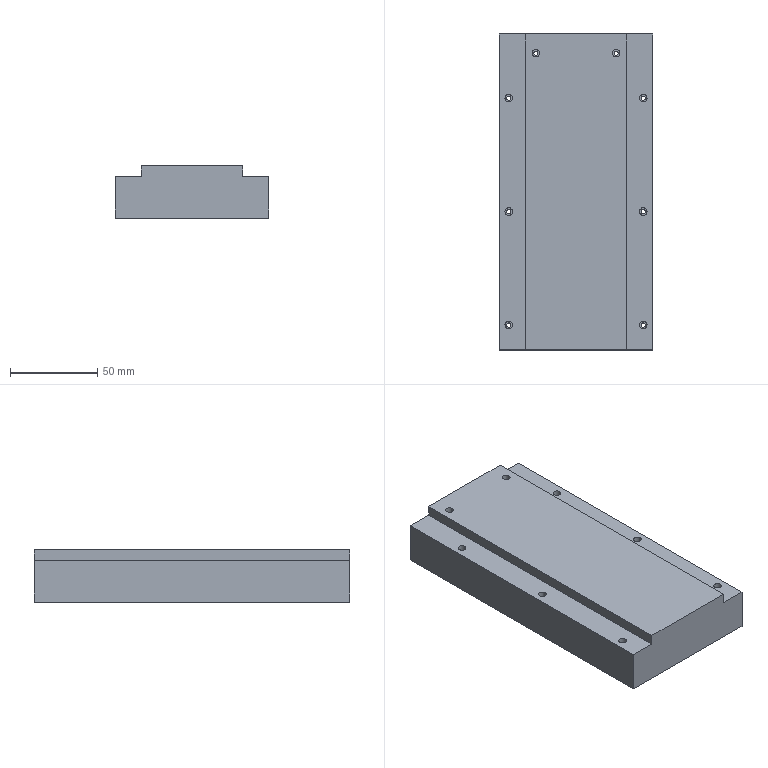NC program | NX | posted with a generic post | part box 88 x 181.05 x 30 mm
Lines 7785 to 7800 of 7800:
(PLANAR_MILL_9_COPY_2 , TOOL : D12-36-D12-120-3T-FINISH)
N15502 T03 M6
N15504 G54
N15506 G17 G0 G90 X-5. Y53.649 B0. C0. S3500 M3
N15508 G43 Z54.5 H3
N15510 Z5.5
N15512 G94 G1 Z2.5 F800.
N15514 Y41.649
N15516 Y-41.649
N15518 Y-53.649
N15520 Z5.5
N15522 G0 Z54.5
N15524 M5
N15526 M2